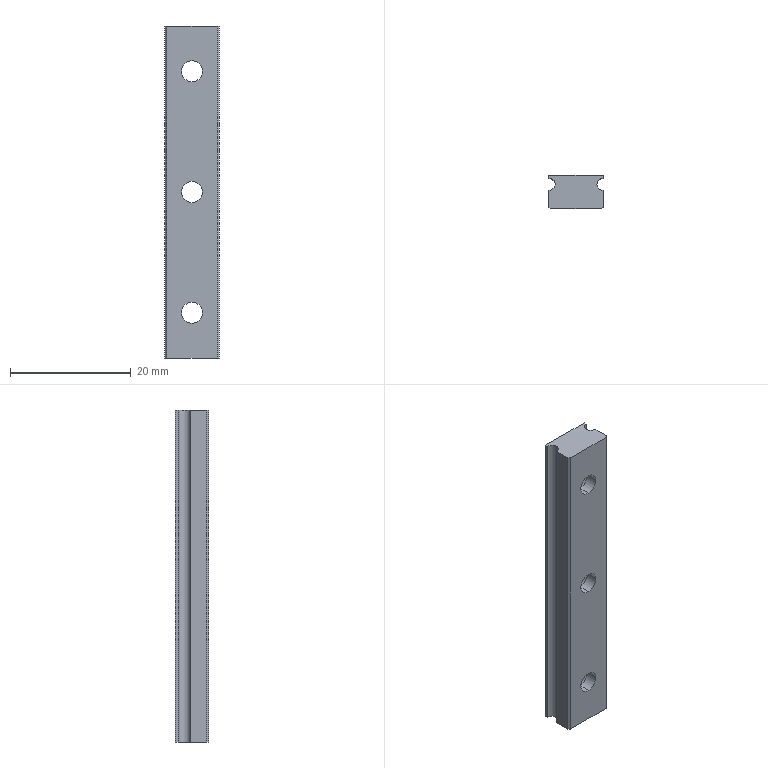Part | STEP file | SEBZ10-551 | 1 solid | 28 faces | box 9 x 5.5 x 55 mm | volume 2176 mm3 | cylinder 15 | plane 13 | commonest cylinder face diameters 3.5 x6 6 x6 2.08 x3